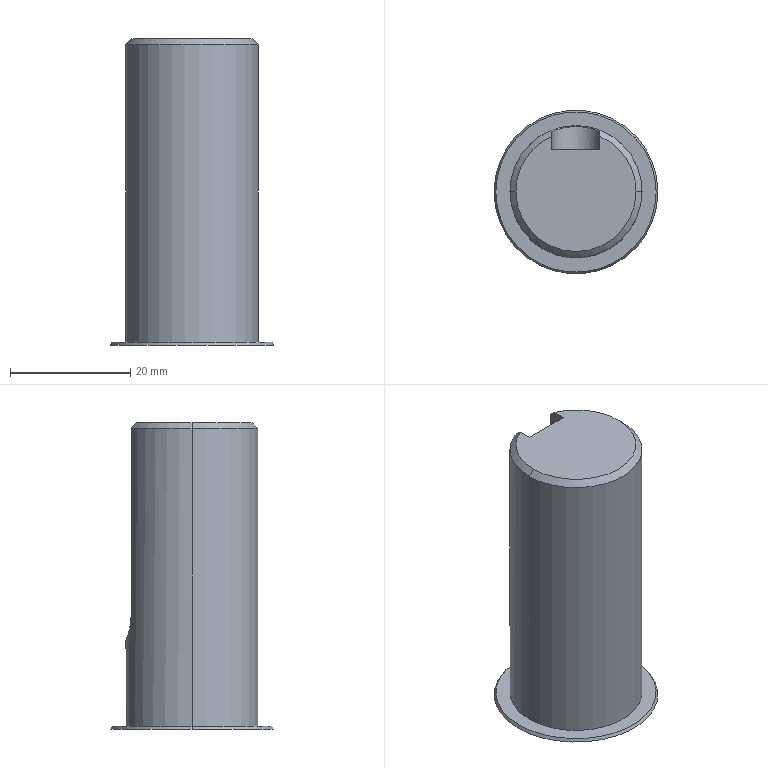Part | STEP file | _1-SOLI00 | 1 solid | 17 faces | box 27.268 x 27.268 x 51 mm | volume 18394 mm3 | plane 8 | cone 5 | cylinder 3 | spline 1 | commonest cylinder face diameters 22 x2 8 x1